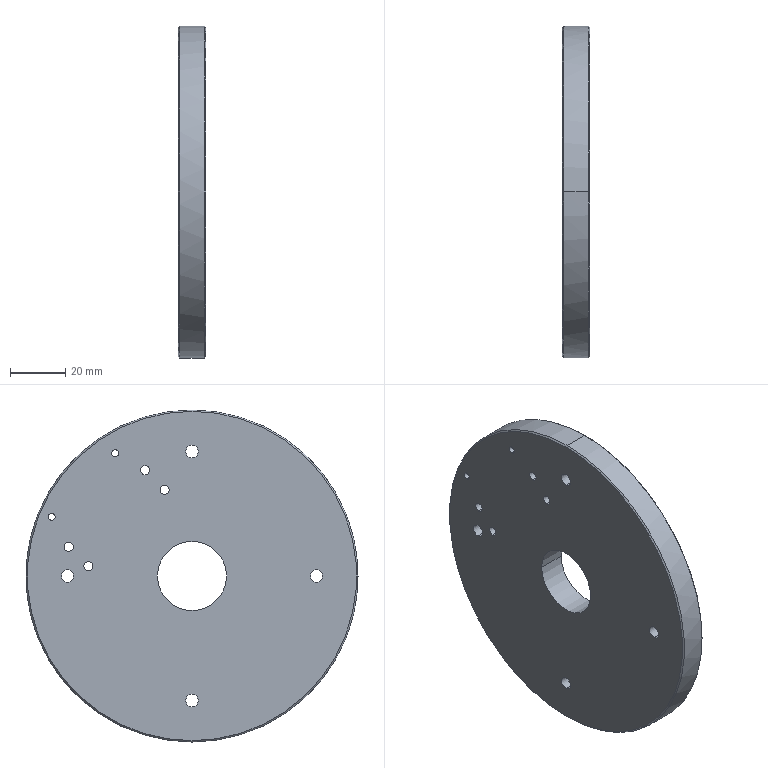Part | STEP file | 06-23 Rotor support plate | 1 solid | 42 faces | box 10 x 120 x 120 mm | volume 106201 mm3 | cylinder 32 | plane 6 | cone 4 | commonest cylinder face diameters 3.3 x8 4.5 x8 8.5 x8 2.5 x4 25 x2 120 x2